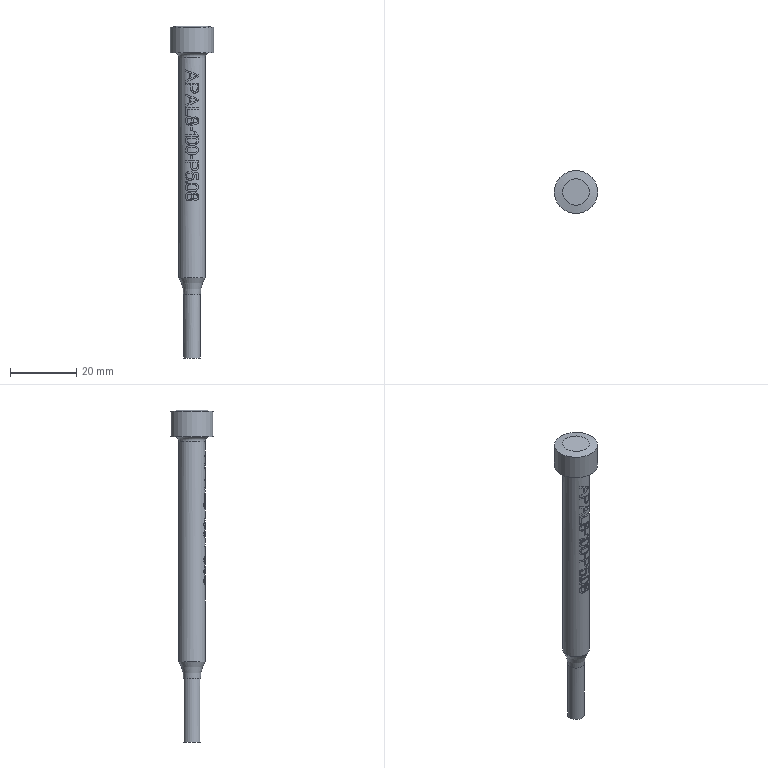Part | STEP file | PN_0051_id1710_x_t | 1 solid | 193 faces | box 13 x 13 x 100 mm | volume 4994 mm3 | plane 110 | cylinder 80 | torus 2 | cone 1 | commonest cylinder face diameters 7.8 x15 8 x12 1.277 x4 1.596 x4 1.671 x3 1.994 x3